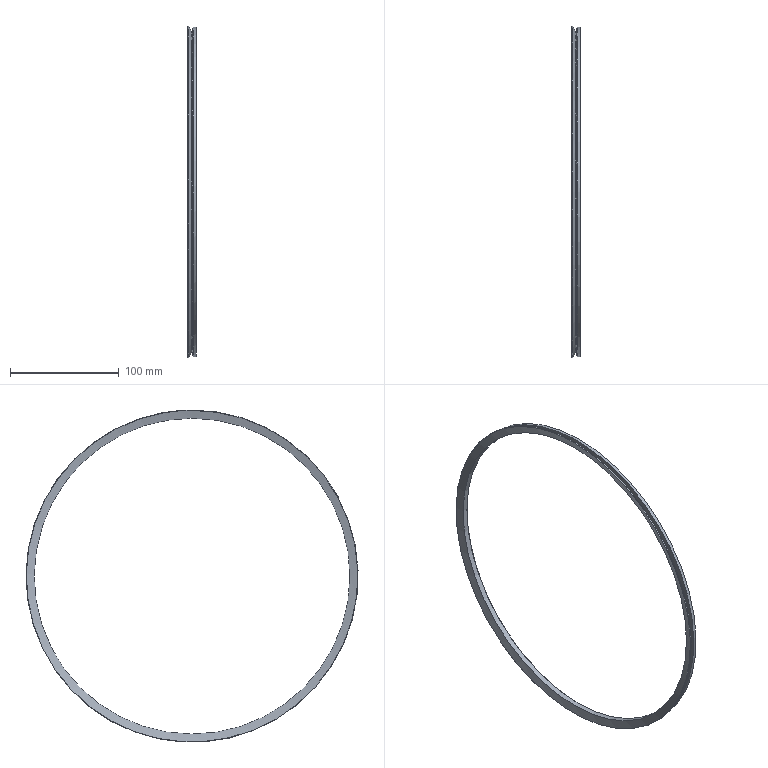Part | STEP file | Part [25] | 1 solid | 9 faces | box 8 x 304.945 x 304.945 mm | volume 31163 mm3 | cone 5 | cylinder 2 | torus 1 | plane 1 | commonest cylinder face diameters 290 x1 303 x1
STEP:
#1=CARTESIAN_POINT('',(4.567,0.,146.546));
#2=VERTEX_POINT('',#1);
#3=CARTESIAN_POINT('',(4.567,146.546,0.));
#4=VERTEX_POINT('',#3);
#5=CARTESIAN_POINT('',(4.567,0.,146.546));
#6=CARTESIAN_POINT('',(4.567,-3.07,146.546));
#7=CARTESIAN_POINT('',(4.567,-9.209,146.353));
#8=CARTESIAN_POINT('',(4.567,-18.382,145.486));
#9=CARTESIAN_POINT('',(4.567,-27.482,144.044));
#10=CARTESIAN_POINT('',(4.567,-36.474,142.034));
#11=CARTESIAN_POINT('',(4.567,-45.322,139.463));
#12=CARTESIAN_POINT('',(4.567,-53.991,136.341));
#13=CARTESIAN_POINT('',(4.567,-62.447,132.682));
#14=CARTESIAN_POINT('',(4.567,-70.656,128.498));
#15=CARTESIAN_POINT('',(4.567,-78.586,123.807));
#16=CARTESIAN_POINT('',(4.567,-86.206,118.628));
#17=CARTESIAN_POINT('',(4.567,-93.486,112.98));
#18=CARTESIAN_POINT('',(4.567,-100.397,106.886));
#19=CARTESIAN_POINT('',(4.567,-106.911,100.37));
#20=CARTESIAN_POINT('',(4.567,-113.003,93.458));
#21=CARTESIAN_POINT('',(4.567,-118.649,86.176));
#22=CARTESIAN_POINT('',(4.567,-123.827,78.555));
#23=CARTESIAN_POINT('',(4.567,-128.516,70.624));
#24=CARTESIAN_POINT('',(4.567,-132.697,62.413));
#25=CARTESIAN_POINT('',(4.567,-136.355,53.957));
#26=CARTESIAN_POINT('',(4.567,-139.474,45.287));
#27=CARTESIAN_POINT('',(4.567,-142.043,36.439));
#28=CARTESIAN_POINT('',(4.567,-144.051,27.446));
#29=CARTESIAN_POINT('',(4.567,-145.49,18.346));
#30=CARTESIAN_POINT('',(4.567,-146.354,9.185));
#31=CARTESIAN_POINT('',(4.567,-146.546,3.058));
#32=CARTESIAN_POINT('',(4.567,-146.546,0.));
#33=CARTESIAN_POINT('',(4.567,-146.546,-3.07));
#34=CARTESIAN_POINT('',(4.567,-146.353,-9.209));
#35=CARTESIAN_POINT('',(4.567,-145.486,-18.382));
#36=CARTESIAN_POINT('',(4.567,-144.044,-27.482));
#37=CARTESIAN_POINT('',(4.567,-142.034,-36.474));
#38=CARTESIAN_POINT('',(4.567,-139.463,-45.322));
#39=CARTESIAN_POINT('',(4.567,-136.341,-53.991));
#40=CARTESIAN_POINT('',(4.567,-132.682,-62.447));
#41=CARTESIAN_POINT('',(4.567,-128.498,-70.656));
#42=CARTESIAN_POINT('',(4.567,-123.807,-78.586));
#43=CARTESIAN_POINT('',(4.567,-118.628,-86.206));
#44=CARTESIAN_POINT('',(4.567,-112.98,-93.486));
#45=CARTESIAN_POINT('',(4.567,-106.886,-100.397));
#46=CARTESIAN_POINT('',(4.567,-100.37,-106.911));
#47=CARTESIAN_POINT('',(4.567,-93.458,-113.003));
#48=CARTESIAN_POINT('',(4.567,-86.176,-118.649));
#49=CARTESIAN_POINT('',(4.567,-78.555,-123.827));
#50=CARTESIAN_POINT('',(4.567,-70.624,-128.516));
#51=CARTESIAN_POINT('',(4.567,-62.413,-132.697));
#52=CARTESIAN_POINT('',(4.567,-53.957,-136.355));
#53=CARTESIAN_POINT('',(4.567,-45.287,-139.474));
#54=CARTESIAN_POINT('',(4.567,-36.439,-142.043));
#55=CARTESIAN_POINT('',(4.567,-27.446,-144.051));
#56=CARTESIAN_POINT('',(4.567,-18.346,-145.49));
#57=CARTESIAN_POINT('',(4.567,-9.173,-146.355));
#58=CARTESIAN_POINT('',(4.567,0.03666,-146.642));
#59=CARTESIAN_POINT('',(4.567,9.246,-146.351));
#60=CARTESIAN_POINT('',(4.567,18.418,-145.481));
#61=CARTESIAN_POINT('',(4.567,27.518,-144.037));
#62=CARTESIAN_POINT('',(4.567,36.51,-142.025));
#63=CARTESIAN_POINT('',(4.567,45.357,-139.452));
#64=CARTESIAN_POINT('',(4.567,54.025,-136.328));
#65=CARTESIAN_POINT('',(4.567,62.48,-132.666));
#66=CARTESIAN_POINT('',(4.567,70.688,-128.48));
#67=CARTESIAN_POINT('',(4.567,78.617,-123.788));
#68=CARTESIAN_POINT('',(4.567,86.236,-118.606));
#69=CARTESIAN_POINT('',(4.567,93.514,-112.956));
#70=CARTESIAN_POINT('',(4.567,100.423,-106.861));
#71=CARTESIAN_POINT('',(4.567,106.936,-100.343));
#72=CARTESIAN_POINT('',(4.567,113.026,-93.429));
#73=CARTESIAN_POINT('',(4.567,118.671,-86.147));
#74=CARTESIAN_POINT('',(4.567,123.847,-78.524));
#75=CARTESIAN_POINT('',(4.567,128.533,-70.592));
#76=CARTESIAN_POINT('',(4.567,132.713,-62.38));
#77=CARTESIAN_POINT('',(4.567,136.368,-53.923));
#78=CARTESIAN_POINT('',(4.567,139.486,-45.252));
#79=CARTESIAN_POINT('',(4.567,142.052,-36.403));
#80=CARTESIAN_POINT('',(4.567,144.058,-27.41));
#81=CARTESIAN_POINT('',(4.567,145.495,-18.309));
#82=CARTESIAN_POINT('',(4.567,146.355,-9.16));
#83=CARTESIAN_POINT('',(4.567,146.546,-3.045));
#84=CARTESIAN_POINT('',(4.567,146.546,0.));
#85=B_SPLINE_CURVE_WITH_KNOTS('',3,(#5,#6,#7,#8,#9,#10,#11,#12,#13,#14,#15,#16,#17,#18,#19,#20,#21,#22,#23,#24,#25,#26,#27,#28,#29,#30,#31,#32,#33,#34,#35,#36,#37,#38,#39,#40,#41,#42,#43,#44,#45,#46,#47,#48,#49,#50,#51,#52,#53,#54,#55,#56,#57,#58,#59,#60,#61,#62,#63,#64,#65,#66,#67,#68,#69,#70,#71,#72,#73,#74,#75,#76,#77,#78,#79,#80,#81,#82,#83,#84),.UNSPECIFIED.,.F.,.F.,(4,1,1,1,1,1,1,1,1,1,1,1,1,1,1,1,1,1,1,1,1,1,1,1,1,3,1,1,1,1,1,1,1,1,1,1,1,1,1,1,1,1,1,1,1,1,1,1,1,1,1,1,1,1,1,1,1,1,1,1,1,1,1,1,1,1,1,1,1,1,1,1,1,1,1,4),(0.,0.01334,0.02667,0.04001,0.05334,0.06668,0.08001,0.09335,0.1067,0.12,0.1334,0.1467,0.16,0.1734,0.1867,0.2,0.2134,0.2267,0.24,0.2534,0.2667,0.28,0.2934,0.3067,0.3201,0.3333,0.3467,0.36,0.3733,0.3867,0.4,0.4133,0.4267,0.44,0.4534,0.4667,0.48,0.4934,0.5067,0.52,0.5334,0.5467,0.56,0.5734,0.5867,0.6,0.6134,0.6267,0.64,0.6534,0.6667,0.6801,0.6934,0.7067,0.7201,0.7334,0.7467,0.7601,0.7734,0.7867,0.8001,0.8134,0.8267,0.8401,0.8534,0.8668,0.8801,0.8934,0.9068,0.9201,0.9334,0.9468,0.9601,0.9734,0.9868,1.),.UNSPECIFIED.);
#86=EDGE_CURVE('',#2,#4,#85,.T.);
#87=ORIENTED_EDGE('',*,*,#86,.F.);
#88=CARTESIAN_POINT('',(4.567,0.,0.));
#89=DIRECTION('',(1.,0.,0.));
#90=DIRECTION('',(0.,1.,0.));
#91=AXIS2_PLACEMENT_3D('',#88,#89,#90);
#92=CIRCLE('',#91,146.546);
#93=EDGE_CURVE('',#4,#2,#92,.T.);
#94=ORIENTED_EDGE('',*,*,#93,.F.);
#95=EDGE_LOOP('',(#87,#94));
#96=FACE_BOUND('',#95,.T.);
#97=CARTESIAN_POINT('',(3.61,146.39,0.));
#98=VERTEX_POINT('',#97);
#99=CARTESIAN_POINT('',(3.61,0.,146.39));
#100=VERTEX_POINT('',#99);
#101=CARTESIAN_POINT('',(3.61,0.,0.));
#102=DIRECTION('',(1.,0.,0.));
#103=DIRECTION('',(0.,1.,0.));
#104=AXIS2_PLACEMENT_3D('',#101,#102,#103);
#105=CIRCLE('',#104,146.39);
#106=EDGE_CURVE('',#98,#100,#105,.T.);
#107=ORIENTED_EDGE('',*,*,#106,.T.);
#108=CARTESIAN_POINT('',(3.61,0.,146.39));
#109=CARTESIAN_POINT('',(3.61,-3.066,146.39));
#110=CARTESIAN_POINT('',(3.61,-9.199,146.197));
#111=CARTESIAN_POINT('',(3.61,-18.363,145.331));
#112=CARTESIAN_POINT('',(3.61,-27.453,143.891));
#113=CARTESIAN_POINT('',(3.61,-36.435,141.883));
#114=CARTESIAN_POINT('',(3.61,-45.274,139.315));
#115=CARTESIAN_POINT('',(3.61,-53.933,136.196));
#116=CARTESIAN_POINT('',(3.61,-62.38,132.541));
#117=CARTESIAN_POINT('',(3.61,-70.581,128.361));
#118=CARTESIAN_POINT('',(3.61,-78.503,123.676));
#119=CARTESIAN_POINT('',(3.61,-86.114,118.501));
#120=CARTESIAN_POINT('',(3.61,-93.386,112.859));
#121=CARTESIAN_POINT('',(3.61,-100.29,106.772));
#122=CARTESIAN_POINT('',(3.61,-106.797,100.263));
#123=CARTESIAN_POINT('',(3.61,-112.883,93.358));
#124=CARTESIAN_POINT('',(3.61,-118.523,86.085));
#125=CARTESIAN_POINT('',(3.61,-123.695,78.472));
#126=CARTESIAN_POINT('',(3.61,-128.379,70.549));
#127=CARTESIAN_POINT('',(3.61,-132.556,62.347));
#128=CARTESIAN_POINT('',(3.61,-136.21,53.899));
#129=CARTESIAN_POINT('',(3.61,-139.326,45.239));
#130=CARTESIAN_POINT('',(3.61,-141.892,36.4));
#131=CARTESIAN_POINT('',(3.61,-143.898,27.417));
#132=CARTESIAN_POINT('',(3.61,-145.336,18.326));
#133=CARTESIAN_POINT('',(3.61,-146.2,9.163));
#134=CARTESIAN_POINT('',(3.61,-146.486,-0.03662));
#135=CARTESIAN_POINT('',(3.61,-146.195,-9.236));
#136=CARTESIAN_POINT('',(3.61,-145.326,-18.399));
#137=CARTESIAN_POINT('',(3.61,-143.884,-27.489));
#138=CARTESIAN_POINT('',(3.61,-141.874,-36.471));
#139=CARTESIAN_POINT('',(3.61,-139.303,-45.309));
#140=CARTESIAN_POINT('',(3.61,-136.183,-53.967));
#141=CARTESIAN_POINT('',(3.61,-132.525,-62.413));
#142=CARTESIAN_POINT('',(3.61,-128.344,-70.613));
#143=CARTESIAN_POINT('',(3.61,-123.656,-78.533));
#144=CARTESIAN_POINT('',(3.61,-118.48,-86.144));
#145=CARTESIAN_POINT('',(3.61,-112.836,-93.415));
#146=CARTESIAN_POINT('',(3.61,-106.747,-100.316));
#147=CARTESIAN_POINT('',(3.61,-100.236,-106.822));
#148=CARTESIAN_POINT('',(3.61,-93.33,-112.906));
#149=CARTESIAN_POINT('',(3.61,-86.055,-118.544));
#150=CARTESIAN_POINT('',(3.61,-78.441,-123.715));
#151=CARTESIAN_POINT('',(3.61,-70.516,-128.397));
#152=CARTESIAN_POINT('',(3.61,-62.314,-132.572));
#153=CARTESIAN_POINT('',(3.61,-53.865,-136.223));
#154=CARTESIAN_POINT('',(3.61,-45.204,-139.337));
#155=CARTESIAN_POINT('',(3.61,-36.364,-141.901));
#156=CARTESIAN_POINT('',(3.61,-27.381,-143.905));
#157=CARTESIAN_POINT('',(3.61,-18.29,-145.34));
#158=CARTESIAN_POINT('',(3.61,-9.151,-146.2));
#159=CARTESIAN_POINT('',(3.61,-3.042,-146.39));
#160=CARTESIAN_POINT('',(3.61,0.,-146.39));
#161=CARTESIAN_POINT('',(3.61,3.066,-146.39));
#162=CARTESIAN_POINT('',(3.61,9.199,-146.197));
#163=CARTESIAN_POINT('',(3.61,18.363,-145.331));
#164=CARTESIAN_POINT('',(3.61,27.453,-143.891));
#165=CARTESIAN_POINT('',(3.61,36.435,-141.883));
#166=CARTESIAN_POINT('',(3.61,45.274,-139.315));
#167=CARTESIAN_POINT('',(3.61,53.933,-136.196));
#168=CARTESIAN_POINT('',(3.61,62.38,-132.541));
#169=CARTESIAN_POINT('',(3.61,70.581,-128.361));
#170=CARTESIAN_POINT('',(3.61,78.503,-123.676));
#171=CARTESIAN_POINT('',(3.61,86.114,-118.501));
#172=CARTESIAN_POINT('',(3.61,93.386,-112.859));
#173=CARTESIAN_POINT('',(3.61,100.29,-106.772));
#174=CARTESIAN_POINT('',(3.61,106.797,-100.263));
#175=CARTESIAN_POINT('',(3.61,112.883,-93.358));
#176=CARTESIAN_POINT('',(3.61,118.523,-86.085));
#177=CARTESIAN_POINT('',(3.61,123.695,-78.472));
#178=CARTESIAN_POINT('',(3.61,128.379,-70.549));
#179=CARTESIAN_POINT('',(3.61,132.556,-62.347));
#180=CARTESIAN_POINT('',(3.61,136.21,-53.899));
#181=CARTESIAN_POINT('',(3.61,139.326,-45.239));
#182=CARTESIAN_POINT('',(3.61,141.892,-36.4));
#183=CARTESIAN_POINT('',(3.61,143.898,-27.417));
#184=CARTESIAN_POINT('',(3.61,145.336,-18.326));
#185=CARTESIAN_POINT('',(3.61,146.198,-9.175));
#186=CARTESIAN_POINT('',(3.61,146.39,-3.054));
#187=CARTESIAN_POINT('',(3.61,146.39,0.));
#188=B_SPLINE_CURVE_WITH_KNOTS('',3,(#108,#109,#110,#111,#112,#113,#114,#115,#116,#117,#118,#119,#120,#121,#122,#123,#124,#125,#126,#127,#128,#129,#130,#131,#132,#133,#134,#135,#136,#137,#138,#139,#140,#141,#142,#143,#144,#145,#146,#147,#148,#149,#150,#151,#152,#153,#154,#155,#156,#157,#158,#159,#160,#161,#162,#163,#164,#165,#166,#167,#168,#169,#170,#171,#172,#173,#174,#175,#176,#177,#178,#179,#180,#181,#182,#183,#184,#185,#186,#187),.UNSPECIFIED.,.F.,.F.,(4,1,1,1,1,1,1,1,1,1,1,1,1,1,1,1,1,1,1,1,1,1,1,1,1,1,1,1,1,1,1,1,1,1,1,1,1,1,1,1,1,1,1,1,1,1,1,1,1,1,3,1,1,1,1,1,1,1,1,1,1,1,1,1,1,1,1,1,1,1,1,1,1,1,1,4),(0.,0.01334,0.02667,0.04001,0.05334,0.06668,0.08001,0.09335,0.1067,0.12,0.1334,0.1467,0.16,0.1734,0.1867,0.2,0.2134,0.2267,0.24,0.2534,0.2667,0.28,0.2934,0.3067,0.3201,0.3334,0.3467,0.3601,0.3734,0.3867,0.4001,0.4134,0.4267,0.4401,0.4534,0.4667,0.4801,0.4934,0.5067,0.5201,0.5334,0.5468,0.5601,0.5734,0.5868,0.6001,0.6134,0.6268,0.6401,0.6534,0.6667,0.68,0.6933,0.7067,0.72,0.7333,0.7467,0.76,0.7734,0.7867,0.8,0.8134,0.8267,0.84,0.8534,0.8667,0.88,0.8934,0.9067,0.92,0.9334,0.9467,0.96,0.9734,0.9867,1.),.UNSPECIFIED.);
#189=EDGE_CURVE('',#100,#98,#188,.T.);
#190=ORIENTED_EDGE('',*,*,#189,.T.);
#191=EDGE_LOOP('',(#107,#190));
#192=FACE_BOUND('',#191,.T.);
#193=CARTESIAN_POINT('',(4.069,0.,0.));
#194=DIRECTION('',(1.,0.,0.));
#195=DIRECTION('',(0.,1.,0.));
#196=AXIS2_PLACEMENT_3D('',#193,#194,#195);
#197=TOROIDAL_SURFACE('',#196,146.59,0.5);
#198=ADVANCED_FACE('',(#96,#192),#197,.F.);
#199=CARTESIAN_POINT('',(8.,0.,146.));
#200=VERTEX_POINT('',#199);
#201=CARTESIAN_POINT('',(8.,0.,0.));
#202=DIRECTION('',(1.,0.,0.));
#203=DIRECTION('',(0.,0.,-1.));
#204=AXIS2_PLACEMENT_3D('',#201,#202,#203);
#205=CIRCLE('',#204,146.);
#206=EDGE_CURVE('',#200,#200,#205,.T.);
#207=ORIENTED_EDGE('',*,*,#206,.T.);
#208=EDGE_LOOP('',(#207));
#209=FACE_OUTER_BOUND('',#208,.T.);
#210=CARTESIAN_POINT('',(7.,0.,145.));
#211=VERTEX_POINT('',#210);
#212=CARTESIAN_POINT('',(7.,0.,145.));
#213=CARTESIAN_POINT('',(7.,-3.037,145.));
#214=CARTESIAN_POINT('',(7.,-9.112,144.809));
#215=CARTESIAN_POINT('',(7.,-18.188,143.951));
#216=CARTESIAN_POINT('',(7.,-27.192,142.525));
#217=CARTESIAN_POINT('',(7.,-36.089,140.536));
#218=CARTESIAN_POINT('',(7.,-44.844,137.992));
#219=CARTESIAN_POINT('',(7.,-53.421,134.903));
#220=CARTESIAN_POINT('',(7.,-61.788,131.282));
#221=CARTESIAN_POINT('',(7.,-69.91,127.143));
#222=CARTESIAN_POINT('',(7.,-77.757,122.501));
#223=CARTESIAN_POINT('',(7.,-85.297,117.376));
#224=CARTESIAN_POINT('',(7.,-92.5,111.788));
#225=CARTESIAN_POINT('',(7.,-99.337,105.758));
#226=CARTESIAN_POINT('',(7.,-105.783,99.311));
#227=CARTESIAN_POINT('',(7.,-111.811,92.472));
#228=CARTESIAN_POINT('',(7.,-117.397,85.267));
#229=CARTESIAN_POINT('',(7.,-122.521,77.726));
#230=CARTESIAN_POINT('',(7.,-127.16,69.879));
#231=CARTESIAN_POINT('',(7.,-131.297,61.755));
#232=CARTESIAN_POINT('',(7.,-134.917,53.388));
#233=CARTESIAN_POINT('',(7.,-138.003,44.809));
#234=CARTESIAN_POINT('',(7.,-140.545,36.054));
#235=CARTESIAN_POINT('',(7.,-142.531,27.157));
#236=CARTESIAN_POINT('',(7.,-143.956,18.152));
#237=CARTESIAN_POINT('',(7.,-144.811,9.076));
#238=CARTESIAN_POINT('',(7.,-145.095,-0.03627));
#239=CARTESIAN_POINT('',(7.,-144.807,-9.148));
#240=CARTESIAN_POINT('',(7.,-143.946,-18.224));
#241=CARTESIAN_POINT('',(7.,-142.518,-27.228));
#242=CARTESIAN_POINT('',(7.,-140.527,-36.125));
#243=CARTESIAN_POINT('',(7.,-137.981,-44.878));
#244=CARTESIAN_POINT('',(7.,-134.89,-53.455));
#245=CARTESIAN_POINT('',(7.,-131.267,-61.821));
#246=CARTESIAN_POINT('',(7.,-127.125,-69.942));
#247=CARTESIAN_POINT('',(7.,-122.482,-77.788));
#248=CARTESIAN_POINT('',(7.,-117.355,-85.326));
#249=CARTESIAN_POINT('',(7.,-111.765,-92.528));
#250=CARTESIAN_POINT('',(7.,-105.733,-99.364));
#251=CARTESIAN_POINT('',(7.,-99.284,-105.808));
#252=CARTESIAN_POINT('',(7.,-92.444,-111.834));
#253=CARTESIAN_POINT('',(7.,-85.238,-117.419));
#254=CARTESIAN_POINT('',(7.,-77.696,-122.54));
#255=CARTESIAN_POINT('',(7.,-69.847,-127.177));
#256=CARTESIAN_POINT('',(7.,-61.722,-131.313));
#257=CARTESIAN_POINT('',(7.,-53.354,-134.93));
#258=CARTESIAN_POINT('',(7.,-44.775,-138.014));
#259=CARTESIAN_POINT('',(7.,-36.019,-140.554));
#260=CARTESIAN_POINT('',(7.,-27.121,-142.538));
#261=CARTESIAN_POINT('',(7.,-18.116,-143.96));
#262=CARTESIAN_POINT('',(7.,-9.064,-144.811));
#263=CARTESIAN_POINT('',(7.,-3.013,-145.));
#264=CARTESIAN_POINT('',(7.,0.,-145.));
#265=CARTESIAN_POINT('',(7.,3.037,-145.));
#266=CARTESIAN_POINT('',(7.,9.112,-144.809));
#267=CARTESIAN_POINT('',(7.,18.188,-143.951));
#268=CARTESIAN_POINT('',(7.,27.192,-142.525));
#269=CARTESIAN_POINT('',(7.,36.089,-140.536));
#270=CARTESIAN_POINT('',(7.,44.844,-137.992));
#271=CARTESIAN_POINT('',(7.,53.421,-134.903));
#272=CARTESIAN_POINT('',(7.,61.788,-131.282));
#273=CARTESIAN_POINT('',(7.,69.91,-127.143));
#274=CARTESIAN_POINT('',(7.,77.757,-122.501));
#275=CARTESIAN_POINT('',(7.,85.297,-117.376));
#276=CARTESIAN_POINT('',(7.,92.5,-111.788));
#277=CARTESIAN_POINT('',(7.,99.337,-105.758));
#278=CARTESIAN_POINT('',(7.,105.783,-99.311));
#279=CARTESIAN_POINT('',(7.,111.811,-92.472));
#280=CARTESIAN_POINT('',(7.,117.397,-85.267));
#281=CARTESIAN_POINT('',(7.,122.521,-77.726));
#282=CARTESIAN_POINT('',(7.,127.16,-69.879));
#283=CARTESIAN_POINT('',(7.,131.297,-61.755));
#284=CARTESIAN_POINT('',(7.,134.917,-53.388));
#285=CARTESIAN_POINT('',(7.,138.003,-44.809));
#286=CARTESIAN_POINT('',(7.,140.545,-36.054));
#287=CARTESIAN_POINT('',(7.,142.531,-27.157));
#288=CARTESIAN_POINT('',(7.,143.956,-18.152));
#289=CARTESIAN_POINT('',(7.,144.811,-9.076));
#290=CARTESIAN_POINT('',(7.,145.095,0.03627));
#291=CARTESIAN_POINT('',(7.,144.807,9.148));
#292=CARTESIAN_POINT('',(7.,143.946,18.224));
#293=CARTESIAN_POINT('',(7.,142.518,27.228));
#294=CARTESIAN_POINT('',(7.,140.527,36.125));
#295=CARTESIAN_POINT('',(7.,137.981,44.878));
#296=CARTESIAN_POINT('',(7.,134.89,53.455));
#297=CARTESIAN_POINT('',(7.,131.267,61.821));
#298=CARTESIAN_POINT('',(7.,127.125,69.942));
#299=CARTESIAN_POINT('',(7.,122.482,77.788));
#300=CARTESIAN_POINT('',(7.,117.355,85.326));
#301=CARTESIAN_POINT('',(7.,111.765,92.528));
#302=CARTESIAN_POINT('',(7.,105.733,99.364));
#303=CARTESIAN_POINT('',(7.,99.284,105.808));
#304=CARTESIAN_POINT('',(7.,92.444,111.834));
#305=CARTESIAN_POINT('',(7.,85.238,117.419));
#306=CARTESIAN_POINT('',(7.,77.696,122.54));
#307=CARTESIAN_POINT('',(7.,69.847,127.177));
#308=CARTESIAN_POINT('',(7.,61.722,131.313));
#309=CARTESIAN_POINT('',(7.,53.354,134.93));
#310=CARTESIAN_POINT('',(7.,44.775,138.014));
#311=CARTESIAN_POINT('',(7.,36.019,140.554));
#312=CARTESIAN_POINT('',(7.,27.121,142.538));
#313=CARTESIAN_POINT('',(7.,18.116,143.96));
#314=CARTESIAN_POINT('',(7.,9.064,144.811));
#315=CARTESIAN_POINT('',(7.,3.013,145.));
#316=CARTESIAN_POINT('',(7.,0.,145.));
#317=B_SPLINE_CURVE_WITH_KNOTS('',3,(#212,#213,#214,#215,#216,#217,#218,#219,#220,#221,#222,#223,#224,#225,#226,#227,#228,#229,#230,#231,#232,#233,#234,#235,#236,#237,#238,#239,#240,#241,#242,#243,#244,#245,#246,#247,#248,#249,#250,#251,#252,#253,#254,#255,#256,#257,#258,#259,#260,#261,#262,#263,#264,#265,#266,#267,#268,#269,#270,#271,#272,#273,#274,#275,#276,#277,#278,#279,#280,#281,#282,#283,#284,#285,#286,#287,#288,#289,#290,#291,#292,#293,#294,#295,#296,#297,#298,#299,#300,#301,#302,#303,#304,#305,#306,#307,#308,#309,#310,#311,#312,#313,#314,#315,#316),.UNSPECIFIED.,.T.,.F.,(4,1,1,1,1,1,1,1,1,1,1,1,1,1,1,1,1,1,1,1,1,1,1,1,1,1,1,1,1,1,1,1,1,1,1,1,1,1,1,1,1,1,1,1,1,1,1,1,1,1,3,1,1,1,1,1,1,1,1,1,1,1,1,1,1,1,1,1,1,1,1,1,1,1,1,1,1,1,1,1,1,1,1,1,1,1,1,1,1,1,1,1,1,1,1,1,1,1,1,1,4),(0.,0.01,0.02,0.03,0.04001,0.05001,0.06001,0.07001,0.08001,0.09001,0.1,0.11,0.12,0.13,0.14,0.15,0.16,0.17,0.18,0.19,0.2,0.21,0.22,0.23,0.24,0.25,0.26,0.27,0.28,0.29,0.3,0.31,0.3201,0.3301,0.3401,0.3501,0.3601,0.3701,0.3801,0.3901,0.4001,0.4101,0.4201,0.4301,0.4401,0.4501,0.4601,0.4701,0.4801,0.4901,0.5,0.51,0.52,0.53,0.54,0.55,0.56,0.57,0.58,0.59,0.6,0.61,0.62,0.63,0.64,0.65,0.66,0.67,0.68,0.69,0.7,0.71,0.72,0.73,0.74,0.75,0.76,0.77,0.78,0.79,0.8,0.81,0.8201,0.8301,0.8401,0.8501,0.8601,0.8701,0.8801,0.8901,0.9001,0.9101,0.9201,0.9301,0.9401,0.9501,0.9601,0.9701,0.9801,0.9901,1.),.UNSPECIFIED.);
#318=EDGE_CURVE('',#211,#211,#317,.T.);
#319=ORIENTED_EDGE('',*,*,#318,.F.);
#320=EDGE_LOOP('',(#319));
#321=FACE_OUTER_BOUND('',#320,.T.);
#322=CARTESIAN_POINT('',(7.5,0.,0.));
#323=DIRECTION('',(1.,0.,0.));
#324=DIRECTION('',(0.,0.,1.));
#325=AXIS2_PLACEMENT_3D('',#322,#323,#324);
#326=CONICAL_SURFACE('',#325,145.5,0.7854);
#327=ADVANCED_FACE('',(#209,#321),#326,.F.);
#328=CARTESIAN_POINT('',(8.,0.,151.5));
#329=VERTEX_POINT('',#328);
#330=CARTESIAN_POINT('',(8.,0.,0.));
#331=DIRECTION('',(1.,0.,0.));
#332=DIRECTION('',(0.,0.,1.));
#333=AXIS2_PLACEMENT_3D('',#330,#331,#332);
#334=CIRCLE('',#333,151.5);
#335=EDGE_CURVE('',#329,#329,#334,.T.);
#336=ORIENTED_EDGE('',*,*,#335,.F.);
#337=EDGE_LOOP('',(#336));
#338=FACE_OUTER_BOUND('',#337,.T.);
#339=CARTESIAN_POINT('',(5.,0.,151.5));
#340=VERTEX_POINT('',#339);
#341=CARTESIAN_POINT('',(5.,0.,151.5));
#342=CARTESIAN_POINT('',(5.,-3.174,151.5));
#343=CARTESIAN_POINT('',(5.,-9.521,151.3));
#344=CARTESIAN_POINT('',(5.,-19.003,150.404));
#345=CARTESIAN_POINT('',(5.,-28.411,148.914));
#346=CARTESIAN_POINT('',(5.,-37.707,146.835));
#347=CARTESIAN_POINT('',(5.,-46.854,144.178));
#348=CARTESIAN_POINT('',(5.,-55.816,140.951));
#349=CARTESIAN_POINT('',(5.,-64.558,137.167));
#350=CARTESIAN_POINT('',(5.,-73.044,132.842));
#351=CARTESIAN_POINT('',(5.,-81.243,127.993));
#352=CARTESIAN_POINT('',(5.,-89.12,122.638));
#353=CARTESIAN_POINT('',(5.,-96.646,116.799));
#354=CARTESIAN_POINT('',(5.,-103.79,110.499));
#355=CARTESIAN_POINT('',(5.,-110.525,103.763));
#356=CARTESIAN_POINT('',(5.,-116.823,96.617));
#357=CARTESIAN_POINT('',(5.,-122.66,89.09));
#358=CARTESIAN_POINT('',(5.,-128.013,81.211));
#359=CARTESIAN_POINT('',(5.,-132.86,73.011));
#360=CARTESIAN_POINT('',(5.,-137.183,64.523));
#361=CARTESIAN_POINT('',(5.,-140.964,55.781));
#362=CARTESIAN_POINT('',(5.,-144.189,46.818));
#363=CARTESIAN_POINT('',(5.,-146.845,37.67));
#364=CARTESIAN_POINT('',(5.,-148.921,28.374));
#365=CARTESIAN_POINT('',(5.,-150.409,18.966));
#366=CARTESIAN_POINT('',(5.,-151.303,9.483));
#367=CARTESIAN_POINT('',(5.,-151.6,-0.0379));
#368=CARTESIAN_POINT('',(5.,-151.298,-9.558));
#369=CARTESIAN_POINT('',(5.,-150.399,-19.041));
#370=CARTESIAN_POINT('',(5.,-148.907,-28.449));
#371=CARTESIAN_POINT('',(5.,-146.826,-37.744));
#372=CARTESIAN_POINT('',(5.,-144.166,-46.89));
#373=CARTESIAN_POINT('',(5.,-140.937,-55.851));
#374=CARTESIAN_POINT('',(5.,-137.151,-64.592));
#375=CARTESIAN_POINT('',(5.,-132.824,-73.078));
#376=CARTESIAN_POINT('',(5.,-127.972,-81.275));
#377=CARTESIAN_POINT('',(5.,-122.616,-89.151));
#378=CARTESIAN_POINT('',(5.,-116.775,-96.675));
#379=CARTESIAN_POINT('',(5.,-110.473,-103.818));
#380=CARTESIAN_POINT('',(5.,-103.735,-110.551));
#381=CARTESIAN_POINT('',(5.,-96.588,-116.847));
#382=CARTESIAN_POINT('',(5.,-89.059,-122.682));
#383=CARTESIAN_POINT('',(5.,-81.179,-128.033));
#384=CARTESIAN_POINT('',(5.,-72.978,-132.879));
#385=CARTESIAN_POINT('',(5.,-64.489,-137.199));
#386=CARTESIAN_POINT('',(5.,-55.746,-140.978));
#387=CARTESIAN_POINT('',(5.,-46.782,-144.201));
#388=CARTESIAN_POINT('',(5.,-37.634,-146.854));
#389=CARTESIAN_POINT('',(5.,-28.337,-148.928));
#390=CARTESIAN_POINT('',(5.,-18.928,-150.413));
#391=CARTESIAN_POINT('',(5.,-9.47,-151.303));
#392=CARTESIAN_POINT('',(5.,-3.148,-151.5));
#393=CARTESIAN_POINT('',(5.,0.,-151.5));
#394=CARTESIAN_POINT('',(5.,3.174,-151.5));
#395=CARTESIAN_POINT('',(5.,9.521,-151.3));
#396=CARTESIAN_POINT('',(5.,19.003,-150.404));
#397=CARTESIAN_POINT('',(5.,28.411,-148.914));
#398=CARTESIAN_POINT('',(5.,37.707,-146.835));
#399=CARTESIAN_POINT('',(5.,46.854,-144.178));
#400=CARTESIAN_POINT('',(5.,55.816,-140.951));
#401=CARTESIAN_POINT('',(5.,64.558,-137.167));
#402=CARTESIAN_POINT('',(5.,73.044,-132.842));
#403=CARTESIAN_POINT('',(5.,81.243,-127.993));
#404=CARTESIAN_POINT('',(5.,89.12,-122.638));
#405=CARTESIAN_POINT('',(5.,96.646,-116.799));
#406=CARTESIAN_POINT('',(5.,103.79,-110.499));
#407=CARTESIAN_POINT('',(5.,110.525,-103.763));
#408=CARTESIAN_POINT('',(5.,116.823,-96.617));
#409=CARTESIAN_POINT('',(5.,122.66,-89.09));
#410=CARTESIAN_POINT('',(5.,128.013,-81.211));
#411=CARTESIAN_POINT('',(5.,132.86,-73.011));
#412=CARTESIAN_POINT('',(5.,137.183,-64.523));
#413=CARTESIAN_POINT('',(5.,140.964,-55.781));
#414=CARTESIAN_POINT('',(5.,144.189,-46.818));
#415=CARTESIAN_POINT('',(5.,146.845,-37.67));
#416=CARTESIAN_POINT('',(5.,148.921,-28.374));
#417=CARTESIAN_POINT('',(5.,150.409,-18.966));
#418=CARTESIAN_POINT('',(5.,151.303,-9.483));
#419=CARTESIAN_POINT('',(5.,151.6,0.0379));
#420=CARTESIAN_POINT('',(5.,151.298,9.558));
#421=CARTESIAN_POINT('',(5.,150.399,19.041));
#422=CARTESIAN_POINT('',(5.,148.907,28.449));
#423=CARTESIAN_POINT('',(5.,146.826,37.744));
#424=CARTESIAN_POINT('',(5.,144.166,46.89));
#425=CARTESIAN_POINT('',(5.,140.937,55.851));
#426=CARTESIAN_POINT('',(5.,137.151,64.592));
#427=CARTESIAN_POINT('',(5.,132.824,73.078));
#428=CARTESIAN_POINT('',(5.,127.972,81.275));
#429=CARTESIAN_POINT('',(5.,122.616,89.151));
#430=CARTESIAN_POINT('',(5.,116.775,96.675));
#431=CARTESIAN_POINT('',(5.,110.473,103.818));
#432=CARTESIAN_POINT('',(5.,103.735,110.551));
#433=CARTESIAN_POINT('',(5.,96.588,116.847));
#434=CARTESIAN_POINT('',(5.,89.059,122.682));
#435=CARTESIAN_POINT('',(5.,81.179,128.033));
#436=CARTESIAN_POINT('',(5.,72.978,132.879));
#437=CARTESIAN_POINT('',(5.,64.489,137.199));
#438=CARTESIAN_POINT('',(5.,55.746,140.978));
#439=CARTESIAN_POINT('',(5.,46.782,144.201));
#440=CARTESIAN_POINT('',(5.,37.634,146.854));
#441=CARTESIAN_POINT('',(5.,28.337,148.928));
#442=CARTESIAN_POINT('',(5.,18.928,150.413));
#443=CARTESIAN_POINT('',(5.,9.47,151.303));
#444=CARTESIAN_POINT('',(5.,3.148,151.5));
#445=CARTESIAN_POINT('',(5.,0.,151.5));
#446=B_SPLINE_CURVE_WITH_KNOTS('',3,(#341,#342,#343,#344,#345,#346,#347,#348,#349,#350,#351,#352,#353,#354,#355,#356,#357,#358,#359,#360,#361,#362,#363,#364,#365,#366,#367,#368,#369,#370,#371,#372,#373,#374,#375,#376,#377,#378,#379,#380,#381,#382,#383,#384,#385,#386,#387,#388,#389,#390,#391,#392,#393,#394,#395,#396,#397,#398,#399,#400,#401,#402,#403,#404,#405,#406,#407,#408,#409,#410,#411,#412,#413,#414,#415,#416,#417,#418,#419,#420,#421,#422,#423,#424,#425,#426,#427,#428,#429,#430,#431,#432,#433,#434,#435,#436,#437,#438,#439,#440,#441,#442,#443,#444,#445),.UNSPECIFIED.,.T.,.F.,(4,1,1,1,1,1,1,1,1,1,1,1,1,1,1,1,1,1,1,1,1,1,1,1,1,1,1,1,1,1,1,1,1,1,1,1,1,1,1,1,1,1,1,1,1,1,1,1,1,1,3,1,1,1,1,1,1,1,1,1,1,1,1,1,1,1,1,1,1,1,1,1,1,1,1,1,1,1,1,1,1,1,1,1,1,1,1,1,1,1,1,1,1,1,1,1,1,1,1,1,4),(0.,0.01,0.02,0.03,0.04001,0.05001,0.06001,0.07001,0.08001,0.09001,0.1,0.11,0.12,0.13,0.14,0.15,0.16,0.17,0.18,0.19,0.2,0.21,0.22,0.23,0.24,0.25,0.26,0.27,0.28,0.29,0.3,0.31,0.3201,0.3301,0.3401,0.3501,0.3601,0.3701,0.3801,0.3901,0.4001,0.4101,0.4201,0.4301,0.4401,0.4501,0.4601,0.4701,0.4801,0.4901,0.5,0.51,0.52,0.53,0.54,0.55,0.56,0.57,0.58,0.59,0.6,0.61,0.62,0.63,0.64,0.65,0.66,0.67,0.68,0.69,0.7,0.71,0.72,0.73,0.74,0.75,0.76,0.77,0.78,0.79,0.8,0.81,0.8201,0.8301,0.8401,0.8501,0.8601,0.8701,0.8801,0.8901,0.9001,0.9101,0.9201,0.9301,0.9401,0.9501,0.9601,0.9701,0.9801,0.9901,1.),.UNSPECIFIED.);
#447=EDGE_CURVE('',#340,#340,#446,.T.);
#448=ORIENTED_EDGE('',*,*,#447,.T.);
#449=EDGE_LOOP('',(#448));
#450=FACE_OUTER_BOUND('',#449,.T.);
#451=CARTESIAN_POINT('',(6.5,0.,0.));
#452=DIRECTION('',(1.,0.,0.));
#453=DIRECTION('',(0.,0.,1.));
#454=AXIS2_PLACEMENT_3D('',#451,#452,#453);
#455=CYLINDRICAL_SURFACE('',#454,151.5);
#456=ADVANCED_FACE('',(#338,#450),#455,.T.);
#457=ORIENTED_EDGE('',*,*,#447,.F.);
#458=EDGE_LOOP('',(#457));
#459=FACE_OUTER_BOUND('',#458,.T.);
#460=ORIENTED_EDGE('',*,*,#93,.T.);
#461=ORIENTED_EDGE('',*,*,#86,.T.);
#462=EDGE_LOOP('',(#460,#461));
#463=FACE_BOUND('',#462,.T.);
#464=CARTESIAN_POINT('',(4.783,0.,0.));
#465=DIRECTION('',(1.,0.,0.));
#466=DIRECTION('',(0.,0.,1.));
#467=AXIS2_PLACEMENT_3D('',#464,#465,#466);
#468=CONICAL_SURFACE('',#467,149.023,1.484);
#469=ADVANCED_FACE('',(#459,#463),#468,.T.);
#470=ORIENTED_EDGE('',*,*,#189,.F.);
#471=ORIENTED_EDGE('',*,*,#106,.F.);
#472=EDGE_LOOP('',(#470,#471));
#473=FACE_BOUND('',#472,.T.);
#474=CARTESIAN_POINT('',(0.9636,0.,152.472));
#475=VERTEX_POINT('',#474);
#476=CARTESIAN_POINT('',(0.9636,0.,152.472));
#477=CARTESIAN_POINT('',(0.9636,-3.194,152.473));
#478=CARTESIAN_POINT('',(0.9636,-9.582,152.272));
#479=CARTESIAN_POINT('',(0.9636,-19.125,151.369));
#480=CARTESIAN_POINT('',(0.9636,-28.594,149.869));
#481=CARTESIAN_POINT('',(0.9636,-37.949,147.778));
#482=CARTESIAN_POINT('',(0.9636,-47.155,145.103));
#483=CARTESIAN_POINT('',(0.9636,-56.174,141.855));
#484=CARTESIAN_POINT('',(0.9636,-64.972,138.047));
#485=CARTESIAN_POINT('',(0.9636,-73.513,133.695));
#486=CARTESIAN_POINT('',(0.9636,-81.764,128.814));
#487=CARTESIAN_POINT('',(0.9636,-89.692,123.425));
#488=CARTESIAN_POINT('',(0.9636,-97.266,117.549));
#489=CARTESIAN_POINT('',(0.9636,-104.457,111.208));
#490=CARTESIAN_POINT('',(0.9636,-111.234,104.429));
#491=CARTESIAN_POINT('',(0.9636,-117.573,97.237));
#492=CARTESIAN_POINT('',(0.9636,-123.447,89.662));
#493=CARTESIAN_POINT('',(0.9636,-128.835,81.732));
#494=CARTESIAN_POINT('',(0.9636,-133.713,73.48));
#495=CARTESIAN_POINT('',(0.9636,-138.064,64.937));
#496=CARTESIAN_POINT('',(0.9636,-141.869,56.139));
#497=CARTESIAN_POINT('',(0.9636,-145.115,47.119));
#498=CARTESIAN_POINT('',(0.9636,-147.787,37.912));
#499=CARTESIAN_POINT('',(0.9636,-149.877,28.556));
#500=CARTESIAN_POINT('',(0.9636,-151.374,19.088));
#501=CARTESIAN_POINT('',(0.9636,-152.274,9.544));
#502=CARTESIAN_POINT('',(0.9636,-152.573,-0.03814));
#503=CARTESIAN_POINT('',(0.9636,-152.269,-9.62));
#504=CARTESIAN_POINT('',(0.9636,-151.365,-19.163));
#505=CARTESIAN_POINT('',(0.9636,-149.862,-28.631));
#506=CARTESIAN_POINT('',(0.9636,-147.768,-37.986));
#507=CARTESIAN_POINT('',(0.9636,-145.091,-47.191));
#508=CARTESIAN_POINT('',(0.9636,-141.841,-56.21));
#509=CARTESIAN_POINT('',(0.9636,-138.031,-65.007));
#510=CARTESIAN_POINT('',(0.9636,-133.676,-73.547));
#511=CARTESIAN_POINT('',(0.9636,-128.794,-81.796));
#512=CARTESIAN_POINT('',(0.9636,-123.403,-89.723));
#513=CARTESIAN_POINT('',(0.9636,-117.524,-97.296));
#514=CARTESIAN_POINT('',(0.9636,-111.182,-104.484));
#515=CARTESIAN_POINT('',(0.9636,-104.401,-111.26));
#516=CARTESIAN_POINT('',(0.9636,-97.208,-117.597));
#517=CARTESIAN_POINT('',(0.9636,-89.631,-123.47));
#518=CARTESIAN_POINT('',(0.9636,-81.7,-128.855));
#519=CARTESIAN_POINT('',(0.9636,-73.446,-133.731));
#520=CARTESIAN_POINT('',(0.9636,-64.903,-138.08));
#521=CARTESIAN_POINT('',(0.9636,-56.103,-141.883));
#522=CARTESIAN_POINT('',(0.9636,-47.082,-145.127));
#523=CARTESIAN_POINT('',(0.9636,-37.875,-147.797));
#524=CARTESIAN_POINT('',(0.9636,-28.519,-149.884));
#525=CARTESIAN_POINT('',(0.9636,-19.05,-151.379));
#526=CARTESIAN_POINT('',(0.9636,-9.531,-152.274));
#527=CARTESIAN_POINT('',(0.9636,-3.168,-152.473));
#528=CARTESIAN_POINT('',(0.9636,0.,-152.472));
#529=CARTESIAN_POINT('',(0.9636,3.194,-152.473));
#530=CARTESIAN_POINT('',(0.9636,9.582,-152.272));
#531=CARTESIAN_POINT('',(0.9636,19.125,-151.369));
#532=CARTESIAN_POINT('',(0.9636,28.594,-149.869));
#533=CARTESIAN_POINT('',(0.9636,37.949,-147.778));
#534=CARTESIAN_POINT('',(0.9636,47.155,-145.103));
#535=CARTESIAN_POINT('',(0.9636,56.174,-141.855));
#536=CARTESIAN_POINT('',(0.9636,64.972,-138.047));
#537=CARTESIAN_POINT('',(0.9636,73.513,-133.695));
#538=CARTESIAN_POINT('',(0.9636,81.764,-128.814));
#539=CARTESIAN_POINT('',(0.9636,89.692,-123.425));
#540=CARTESIAN_POINT('',(0.9636,97.266,-117.549));
#541=CARTESIAN_POINT('',(0.9636,104.457,-111.208));
#542=CARTESIAN_POINT('',(0.9636,111.234,-104.429));
#543=CARTESIAN_POINT('',(0.9636,117.573,-97.237));
#544=CARTESIAN_POINT('',(0.9636,123.447,-89.662));
#545=CARTESIAN_POINT('',(0.9636,128.835,-81.732));
#546=CARTESIAN_POINT('',(0.9636,133.713,-73.48));
#547=CARTESIAN_POINT('',(0.9636,138.064,-64.937));
#548=CARTESIAN_POINT('',(0.9636,141.869,-56.139));
#549=CARTESIAN_POINT('',(0.9636,145.115,-47.119));
#550=CARTESIAN_POINT('',(0.9636,147.787,-37.912));
#551=CARTESIAN_POINT('',(0.9636,149.877,-28.556));
#552=CARTESIAN_POINT('',(0.9636,151.374,-19.088));
#553=CARTESIAN_POINT('',(0.9636,152.274,-9.544));
#554=CARTESIAN_POINT('',(0.9636,152.573,0.03814));
#555=CARTESIAN_POINT('',(0.9636,152.269,9.62));
#556=CARTESIAN_POINT('',(0.9636,151.365,19.163));
#557=CARTESIAN_POINT('',(0.9636,149.862,28.631));
#558=CARTESIAN_POINT('',(0.9636,147.768,37.986));
#559=CARTESIAN_POINT('',(0.9636,145.091,47.191));
#560=CARTESIAN_POINT('',(0.9636,141.841,56.21));
#561=CARTESIAN_POINT('',(0.9636,138.031,65.007));
#562=CARTESIAN_POINT('',(0.9636,133.676,73.547));
#563=CARTESIAN_POINT('',(0.9636,128.794,81.796));
#564=CARTESIAN_POINT('',(0.9636,123.403,89.723));
#565=CARTESIAN_POINT('',(0.9636,117.524,97.296));
#566=CARTESIAN_POINT('',(0.9636,111.182,104.484));
#567=CARTESIAN_POINT('',(0.9636,104.401,111.26));
#568=CARTESIAN_POINT('',(0.9636,97.208,117.597));
#569=CARTESIAN_POINT('',(0.9636,89.631,123.47));
#570=CARTESIAN_POINT('',(0.9636,81.7,128.855));
#571=CARTESIAN_POINT('',(0.9636,73.446,133.731));
#572=CARTESIAN_POINT('',(0.9636,64.903,138.08));
#573=CARTESIAN_POINT('',(0.9636,56.103,141.883));
#574=CARTESIAN_POINT('',(0.9636,47.082,145.127));
#575=CARTESIAN_POINT('',(0.9636,37.875,147.797));
#576=CARTESIAN_POINT('',(0.9636,28.519,149.884));
#577=CARTESIAN_POINT('',(0.9636,19.05,151.379));
#578=CARTESIAN_POINT('',(0.9636,9.531,152.274));
#579=CARTESIAN_POINT('',(0.9636,3.168,152.473));
#580=CARTESIAN_POINT('',(0.9636,0.,152.472));
#581=B_SPLINE_CURVE_WITH_KNOTS('',3,(#476,#477,#478,#479,#480,#481,#482,#483,#484,#485,#486,#487,#488,#489,#490,#491,#492,#493,#494,#495,#496,#497,#498,#499,#500,#501,#502,#503,#504,#505,#506,#507,#508,#509,#510,#511,#512,#513,#514,#515,#516,#517,#518,#519,#520,#521,#522,#523,#524,#525,#526,#527,#528,#529,#530,#531,#532,#533,#534,#535,#536,#537,#538,#539,#540,#541,#542,#543,#544,#545,#546,#547,#548,#549,#550,#551,#552,#553,#554,#555,#556,#557,#558,#559,#560,#561,#562,#563,#564,#565,#566,#567,#568,#569,#570,#571,#572,#573,#574,#575,#576,#577,#578,#579,#580),.UNSPECIFIED.,.T.,.F.,(4,1,1,1,1,1,1,1,1,1,1,1,1,1,1,1,1,1,1,1,1,1,1,1,1,1,1,1,1,1,1,1,1,1,1,1,1,1,1,1,1,1,1,1,1,1,1,1,1,1,3,1,1,1,1,1,1,1,1,1,1,1,1,1,1,1,1,1,1,1,1,1,1,1,1,1,1,1,1,1,1,1,1,1,1,1,1,1,1,1,1,1,1,1,1,1,1,1,1,1,4),(0.,0.01,0.02,0.03,0.04001,0.05001,0.06001,0.07001,0.08001,0.09001,0.1,0.11,0.12,0.13,0.14,0.15,0.16,0.17,0.18,0.19,0.2,0.21,0.22,0.23,0.24,0.25,0.26,0.27,0.28,0.29,0.3,0.31,0.3201,0.3301,0.3401,0.3501,0.3601,0.3701,0.3801,0.3901,0.4001,0.4101,0.4201,0.4301,0.4401,0.4501,0.4601,0.4701,0.4801,0.4901,0.5,0.51,0.52,0.53,0.54,0.55,0.56,0.57,0.58,0.59,0.6,0.61,0.62,0.63,0.64,0.65,0.66,0.67,0.68,0.69,0.7,0.71,0.72,0.73,0.74,0.75,0.76,0.77,0.78,0.79,0.8,0.81,0.8201,0.8301,0.8401,0.8501,0.8601,0.8701,0.8801,0.8901,0.9001,0.9101,0.9201,0.9301,0.9401,0.9501,0.9601,0.9701,0.9801,0.9901,1.),.UNSPECIFIED.);
#582=EDGE_CURVE('',#475,#475,#581,.T.);
#583=ORIENTED_EDGE('',*,*,#582,.T.);
#584=EDGE_LOOP('',(#583));
#585=FACE_OUTER_BOUND('',#584,.T.);
#586=CARTESIAN_POINT('',(2.287,0.,0.));
#587=DIRECTION('',(-1.,0.,0.));
#588=DIRECTION('',(0.,0.,1.));
#589=AXIS2_PLACEMENT_3D('',#586,#587,#588);
#590=CONICAL_SURFACE('',#589,149.431,1.16);
#591=ADVANCED_FACE('',(#473,#585),#590,.T.);
#592=ORIENTED_EDGE('',*,*,#582,.F.);
#593=EDGE_LOOP('',(#592));
#594=FACE_OUTER_BOUND('',#593,.T.);
#595=CARTESIAN_POINT('',(0.,0.,152.205));
#596=VERTEX_POINT('',#595);
#597=CARTESIAN_POINT('',(0.,0.,152.205));
#598=CARTESIAN_POINT('',(0.,-3.188,152.205));
#599=CARTESIAN_POINT('',(0.,-9.565,152.004));
#600=CARTESIAN_POINT('',(0.,-19.092,151.104));
#601=CARTESIAN_POINT('',(0.,-28.544,149.606));
#602=CARTESIAN_POINT('',(0.,-37.883,147.519));
#603=CARTESIAN_POINT('',(0.,-47.072,144.848));
#604=CARTESIAN_POINT('',(0.,-56.076,141.606));
#605=CARTESIAN_POINT('',(0.,-64.858,137.805));
#606=CARTESIAN_POINT('',(0.,-73.384,133.46));
#607=CARTESIAN_POINT('',(0.,-81.621,128.588));
#608=CARTESIAN_POINT('',(0.,-89.535,123.208));
#609=CARTESIAN_POINT('',(0.,-97.096,117.342));
#610=CARTESIAN_POINT('',(0.,-104.273,111.013));
#611=CARTESIAN_POINT('',(0.,-111.039,104.246));
#612=CARTESIAN_POINT('',(0.,-117.367,97.066));
#613=CARTESIAN_POINT('',(0.,-123.231,89.504));
#614=CARTESIAN_POINT('',(0.,-128.609,81.589));
#615=CARTESIAN_POINT('',(0.,-133.478,73.351));
#616=CARTESIAN_POINT('',(0.,-137.821,64.824));
#617=CARTESIAN_POINT('',(0.,-141.62,56.04));
#618=CARTESIAN_POINT('',(0.,-144.86,47.036));
#619=CARTESIAN_POINT('',(0.,-147.528,37.846));
#620=CARTESIAN_POINT('',(0.,-149.614,28.506));
#621=CARTESIAN_POINT('',(0.,-151.109,19.054));
#622=CARTESIAN_POINT('',(0.,-152.007,9.527));
#623=CARTESIAN_POINT('',(0.,-152.305,-0.03808));
#624=CARTESIAN_POINT('',(0.,-152.002,-9.603));
#625=CARTESIAN_POINT('',(0.,-151.099,-19.13));
#626=CARTESIAN_POINT('',(0.,-149.599,-28.581));
#627=CARTESIAN_POINT('',(0.,-147.509,-37.92));
#628=CARTESIAN_POINT('',(0.,-144.837,-47.108));
#629=CARTESIAN_POINT('',(0.,-141.592,-56.111));
#630=CARTESIAN_POINT('',(0.,-137.789,-64.892));
#631=CARTESIAN_POINT('',(0.,-133.442,-73.418));
#632=CARTESIAN_POINT('',(0.,-128.568,-81.653));
#633=CARTESIAN_POINT('',(0.,-123.186,-89.566));
#634=CARTESIAN_POINT('',(0.,-117.318,-97.125));
#635=CARTESIAN_POINT('',(0.,-110.987,-104.301));
#636=CARTESIAN_POINT('',(0.,-104.218,-111.065));
#637=CARTESIAN_POINT('',(0.,-97.037,-117.391));
#638=CARTESIAN_POINT('',(0.,-89.473,-123.253));
#639=CARTESIAN_POINT('',(0.,-81.556,-128.629));
#640=CARTESIAN_POINT('',(0.,-73.317,-133.497));
#641=CARTESIAN_POINT('',(0.,-64.789,-137.838));
#642=CARTESIAN_POINT('',(0.,-56.005,-141.634));
#643=CARTESIAN_POINT('',(0.,-47.,-144.872));
#644=CARTESIAN_POINT('',(0.,-37.809,-147.538));
#645=CARTESIAN_POINT('',(0.,-28.469,-149.621));
#646=CARTESIAN_POINT('',(0.,-19.016,-151.113));
#647=CARTESIAN_POINT('',(0.,-9.514,-152.007));
#648=CARTESIAN_POINT('',(0.,-3.163,-152.205));
#649=CARTESIAN_POINT('',(0.,0.,-152.205));
#650=CARTESIAN_POINT('',(0.,3.188,-152.205));
#651=CARTESIAN_POINT('',(0.,9.565,-152.004));
#652=CARTESIAN_POINT('',(0.,19.092,-151.104));
#653=CARTESIAN_POINT('',(0.,28.544,-149.606));
#654=CARTESIAN_POINT('',(0.,37.883,-147.519));
#655=CARTESIAN_POINT('',(0.,47.072,-144.848));
#656=CARTESIAN_POINT('',(0.,56.076,-141.606));
#657=CARTESIAN_POINT('',(0.,64.858,-137.805));
#658=CARTESIAN_POINT('',(0.,73.384,-133.46));
#659=CARTESIAN_POINT('',(0.,81.621,-128.588));
#660=CARTESIAN_POINT('',(0.,89.535,-123.208));
#661=CARTESIAN_POINT('',(0.,97.096,-117.342));
#662=CARTESIAN_POINT('',(0.,104.273,-111.013));
#663=CARTESIAN_POINT('',(0.,111.039,-104.246));
#664=CARTESIAN_POINT('',(0.,117.367,-97.066));
#665=CARTESIAN_POINT('',(0.,123.231,-89.504));
#666=CARTESIAN_POINT('',(0.,128.609,-81.589));
#667=CARTESIAN_POINT('',(0.,133.478,-73.351));
#668=CARTESIAN_POINT('',(0.,137.821,-64.824));
#669=CARTESIAN_POINT('',(0.,141.62,-56.04));
#670=CARTESIAN_POINT('',(0.,144.86,-47.036));
#671=CARTESIAN_POINT('',(0.,147.528,-37.846));
#672=CARTESIAN_POINT('',(0.,149.614,-28.506));
#673=CARTESIAN_POINT('',(0.,151.109,-19.054));
#674=CARTESIAN_POINT('',(0.,152.007,-9.527));
#675=CARTESIAN_POINT('',(0.,152.305,0.03808));
#676=CARTESIAN_POINT('',(0.,152.002,9.603));
#677=CARTESIAN_POINT('',(0.,151.099,19.13));
#678=CARTESIAN_POINT('',(0.,149.599,28.581));
#679=CARTESIAN_POINT('',(0.,147.509,37.92));
#680=CARTESIAN_POINT('',(0.,144.837,47.108));
#681=CARTESIAN_POINT('',(0.,141.592,56.111));
#682=CARTESIAN_POINT('',(0.,137.789,64.892));
#683=CARTESIAN_POINT('',(0.,133.442,73.418));
#684=CARTESIAN_POINT('',(0.,128.568,81.653));
#685=CARTESIAN_POINT('',(0.,123.186,89.566));
#686=CARTESIAN_POINT('',(0.,117.318,97.125));
#687=CARTESIAN_POINT('',(0.,110.987,104.301));
#688=CARTESIAN_POINT('',(0.,104.218,111.065));
#689=CARTESIAN_POINT('',(0.,97.037,117.391));
#690=CARTESIAN_POINT('',(0.,89.473,123.253));
#691=CARTESIAN_POINT('',(0.,81.556,128.629));
#692=CARTESIAN_POINT('',(0.,73.317,133.497));
#693=CARTESIAN_POINT('',(0.,64.789,137.838));
#694=CARTESIAN_POINT('',(0.,56.005,141.634));
#695=CARTESIAN_POINT('',(0.,47.,144.872));
#696=CARTESIAN_POINT('',(0.,37.809,147.538));
#697=CARTESIAN_POINT('',(0.,28.469,149.621));
#698=CARTESIAN_POINT('',(0.,19.016,151.113));
#699=CARTESIAN_POINT('',(0.,9.514,152.007));
#700=CARTESIAN_POINT('',(0.,3.163,152.205));
#701=CARTESIAN_POINT('',(0.,0.,152.205));
#702=B_SPLINE_CURVE_WITH_KNOTS('',3,(#597,#598,#599,#600,#601,#602,#603,#604,#605,#606,#607,#608,#609,#610,#611,#612,#613,#614,#615,#616,#617,#618,#619,#620,#621,#622,#623,#624,#625,#626,#627,#628,#629,#630,#631,#632,#633,#634,#635,#636,#637,#638,#639,#640,#641,#642,#643,#644,#645,#646,#647,#648,#649,#650,#651,#652,#653,#654,#655,#656,#657,#658,#659,#660,#661,#662,#663,#664,#665,#666,#667,#668,#669,#670,#671,#672,#673,#674,#675,#676,#677,#678,#679,#680,#681,#682,#683,#684,#685,#686,#687,#688,#689,#690,#691,#692,#693,#694,#695,#696,#697,#698,#699,#700,#701),.UNSPECIFIED.,.T.,.F.,(4,1,1,1,1,1,1,1,1,1,1,1,1,1,1,1,1,1,1,1,1,1,1,1,1,1,1,1,1,1,1,1,1,1,1,1,1,1,1,1,1,1,1,1,1,1,1,1,1,1,3,1,1,1,1,1,1,1,1,1,1,1,1,1,1,1,1,1,1,1,1,1,1,1,1,1,1,1,1,1,1,1,1,1,1,1,1,1,1,1,1,1,1,1,1,1,1,1,1,1,4),(0.,0.01,0.02,0.03,0.04001,0.05001,0.06001,0.07001,0.08001,0.09001,0.1,0.11,0.12,0.13,0.14,0.15,0.16,0.17,0.18,0.19,0.2,0.21,0.22,0.23,0.24,0.25,0.26,0.27,0.28,0.29,0.3,0.31,0.3201,0.3301,0.3401,0.3501,0.3601,0.3701,0.3801,0.3901,0.4001,0.4101,0.4201,0.4301,0.4401,0.4501,0.4601,0.4701,0.4801,0.4901,0.5,0.51,0.52,0.53,0.54,0.55,0.56,0.57,0.58,0.59,0.6,0.61,0.62,0.63,0.64,0.65,0.66,0.67,0.68,0.69,0.7,0.71,0.72,0.73,0.74,0.75,0.76,0.77,0.78,0.79,0.8,0.81,0.8201,0.8301,0.8401,0.8501,0.8601,0.8701,0.8801,0.8901,0.9001,0.9101,0.9201,0.9301,0.9401,0.9501,0.9601,0.9701,0.9801,0.9901,1.),.UNSPECIFIED.);
#703=EDGE_CURVE('',#596,#596,#702,.T.);
#704=ORIENTED_EDGE('',*,*,#703,.T.);
#705=EDGE_LOOP('',(#704));
#706=FACE_OUTER_BOUND('',#705,.T.);
#707=CARTESIAN_POINT('',(0.4818,0.,0.));
#708=DIRECTION('',(1.,0.,0.));
#709=DIRECTION('',(0.,0.,1.));
#710=AXIS2_PLACEMENT_3D('',#707,#708,#709);
#711=CONICAL_SURFACE('',#710,152.339,0.2708);
#712=ADVANCED_FACE('',(#594,#706),#711,.T.);
#713=CARTESIAN_POINT('',(2.,0.,145.));
#714=VERTEX_POINT('',#713);
#715=CARTESIAN_POINT('',(2.,0.,145.));
#716=CARTESIAN_POINT('',(2.,-3.037,145.));
#717=CARTESIAN_POINT('',(2.,-9.112,144.809));
#718=CARTESIAN_POINT('',(2.,-18.188,143.951));
#719=CARTESIAN_POINT('',(2.,-27.192,142.525));
#720=CARTESIAN_POINT('',(2.,-36.089,140.536));
#721=CARTESIAN_POINT('',(2.,-44.844,137.992));
#722=CARTESIAN_POINT('',(2.,-53.421,134.903));
#723=CARTESIAN_POINT('',(2.,-61.788,131.282));
#724=CARTESIAN_POINT('',(2.,-69.91,127.143));
#725=CARTESIAN_POINT('',(2.,-77.757,122.501));
#726=CARTESIAN_POINT('',(2.,-85.297,117.376));
#727=CARTESIAN_POINT('',(2.,-92.5,111.788));
#728=CARTESIAN_POINT('',(2.,-99.337,105.758));
#729=CARTESIAN_POINT('',(2.,-105.783,99.311));
#730=CARTESIAN_POINT('',(2.,-111.811,92.472));
#731=CARTESIAN_POINT('',(2.,-117.397,85.267));
#732=CARTESIAN_POINT('',(2.,-122.521,77.726));
#733=CARTESIAN_POINT('',(2.,-127.16,69.879));
#734=CARTESIAN_POINT('',(2.,-131.297,61.755));
#735=CARTESIAN_POINT('',(2.,-134.917,53.388));
#736=CARTESIAN_POINT('',(2.,-138.003,44.809));
#737=CARTESIAN_POINT('',(2.,-140.545,36.054));
#738=CARTESIAN_POINT('',(2.,-142.531,27.157));
#739=CARTESIAN_POINT('',(2.,-143.956,18.152));
#740=CARTESIAN_POINT('',(2.,-144.811,9.076));
#741=CARTESIAN_POINT('',(2.,-145.095,-0.03627));
#742=CARTESIAN_POINT('',(2.,-144.807,-9.148));
#743=CARTESIAN_POINT('',(2.,-143.946,-18.224));
#744=CARTESIAN_POINT('',(2.,-142.518,-27.228));
#745=CARTESIAN_POINT('',(2.,-140.527,-36.125));
#746=CARTESIAN_POINT('',(2.,-137.981,-44.878));
#747=CARTESIAN_POINT('',(2.,-134.89,-53.455));
#748=CARTESIAN_POINT('',(2.,-131.267,-61.821));
#749=CARTESIAN_POINT('',(2.,-127.125,-69.942));
#750=CARTESIAN_POINT('',(2.,-122.482,-77.788));
#751=CARTESIAN_POINT('',(2.,-117.355,-85.326));
#752=CARTESIAN_POINT('',(2.,-111.765,-92.528));
#753=CARTESIAN_POINT('',(2.,-105.733,-99.364));
#754=CARTESIAN_POINT('',(2.,-99.284,-105.808));
#755=CARTESIAN_POINT('',(2.,-92.444,-111.834));
#756=CARTESIAN_POINT('',(2.,-85.238,-117.419));
#757=CARTESIAN_POINT('',(2.,-77.696,-122.54));
#758=CARTESIAN_POINT('',(2.,-69.847,-127.177));
#759=CARTESIAN_POINT('',(2.,-61.722,-131.313));
#760=CARTESIAN_POINT('',(2.,-53.354,-134.93));
#761=CARTESIAN_POINT('',(2.,-44.775,-138.014));
#762=CARTESIAN_POINT('',(2.,-36.019,-140.554));
#763=CARTESIAN_POINT('',(2.,-27.121,-142.538));
#764=CARTESIAN_POINT('',(2.,-18.116,-143.96));
#765=CARTESIAN_POINT('',(2.,-9.064,-144.811));
#766=CARTESIAN_POINT('',(2.,-3.013,-145.));
#767=CARTESIAN_POINT('',(2.,0.,-145.));
#768=CARTESIAN_POINT('',(2.,3.037,-145.));
#769=CARTESIAN_POINT('',(2.,9.112,-144.809));
#770=CARTESIAN_POINT('',(2.,18.188,-143.951));
#771=CARTESIAN_POINT('',(2.,27.192,-142.525));
#772=CARTESIAN_POINT('',(2.,36.089,-140.536));
#773=CARTESIAN_POINT('',(2.,44.844,-137.992));
#774=CARTESIAN_POINT('',(2.,53.421,-134.903));
#775=CARTESIAN_POINT('',(2.,61.788,-131.282));
#776=CARTESIAN_POINT('',(2.,69.91,-127.143));
#777=CARTESIAN_POINT('',(2.,77.757,-122.501));
#778=CARTESIAN_POINT('',(2.,85.297,-117.376));
#779=CARTESIAN_POINT('',(2.,92.5,-111.788));
#780=CARTESIAN_POINT('',(2.,99.337,-105.758));
#781=CARTESIAN_POINT('',(2.,105.783,-99.311));
#782=CARTESIAN_POINT('',(2.,111.811,-92.472));
#783=CARTESIAN_POINT('',(2.,117.397,-85.267));
#784=CARTESIAN_POINT('',(2.,122.521,-77.726));
#785=CARTESIAN_POINT('',(2.,127.16,-69.879));
#786=CARTESIAN_POINT('',(2.,131.297,-61.755));
#787=CARTESIAN_POINT('',(2.,134.917,-53.388));
#788=CARTESIAN_POINT('',(2.,138.003,-44.809));
#789=CARTESIAN_POINT('',(2.,140.545,-36.054));
#790=CARTESIAN_POINT('',(2.,142.531,-27.157));
#791=CARTESIAN_POINT('',(2.,143.956,-18.152));
#792=CARTESIAN_POINT('',(2.,144.811,-9.076));
#793=CARTESIAN_POINT('',(2.,145.095,0.03627));
#794=CARTESIAN_POINT('',(2.,144.807,9.148));
#795=CARTESIAN_POINT('',(2.,143.946,18.224));
#796=CARTESIAN_POINT('',(2.,142.518,27.228));
#797=CARTESIAN_POINT('',(2.,140.527,36.125));
#798=CARTESIAN_POINT('',(2.,137.981,44.878));
#799=CARTESIAN_POINT('',(2.,134.89,53.455));
#800=CARTESIAN_POINT('',(2.,131.267,61.821));
#801=CARTESIAN_POINT('',(2.,127.125,69.942));
#802=CARTESIAN_POINT('',(2.,122.482,77.788));
#803=CARTESIAN_POINT('',(2.,117.355,85.326));
#804=CARTESIAN_POINT('',(2.,111.765,92.528));
#805=CARTESIAN_POINT('',(2.,105.733,99.364));
#806=CARTESIAN_POINT('',(2.,99.284,105.808));
#807=CARTESIAN_POINT('',(2.,92.444,111.834));
#808=CARTESIAN_POINT('',(2.,85.238,117.419));
#809=CARTESIAN_POINT('',(2.,77.696,122.54));
#810=CARTESIAN_POINT('',(2.,69.847,127.177));
#811=CARTESIAN_POINT('',(2.,61.722,131.313));
#812=CARTESIAN_POINT('',(2.,53.354,134.93));
#813=CARTESIAN_POINT('',(2.,44.775,138.014));
#814=CARTESIAN_POINT('',(2.,36.019,140.554));
#815=CARTESIAN_POINT('',(2.,27.121,142.538));
#816=CARTESIAN_POINT('',(2.,18.116,143.96));
#817=CARTESIAN_POINT('',(2.,9.064,144.811));
#818=CARTESIAN_POINT('',(2.,3.013,145.));
#819=CARTESIAN_POINT('',(2.,0.,145.));
#820=B_SPLINE_CURVE_WITH_KNOTS('',3,(#715,#716,#717,#718,#719,#720,#721,#722,#723,#724,#725,#726,#727,#728,#729,#730,#731,#732,#733,#734,#735,#736,#737,#738,#739,#740,#741,#742,#743,#744,#745,#746,#747,#748,#749,#750,#751,#752,#753,#754,#755,#756,#757,#758,#759,#760,#761,#762,#763,#764,#765,#766,#767,#768,#769,#770,#771,#772,#773,#774,#775,#776,#777,#778,#779,#780,#781,#782,#783,#784,#785,#786,#787,#788,#789,#790,#791,#792,#793,#794,#795,#796,#797,#798,#799,#800,#801,#802,#803,#804,#805,#806,#807,#808,#809,#810,#811,#812,#813,#814,#815,#816,#817,#818,#819),.UNSPECIFIED.,.T.,.F.,(4,1,1,1,1,1,1,1,1,1,1,1,1,1,1,1,1,1,1,1,1,1,1,1,1,1,1,1,1,1,1,1,1,1,1,1,1,1,1,1,1,1,1,1,1,1,1,1,1,1,3,1,1,1,1,1,1,1,1,1,1,1,1,1,1,1,1,1,1,1,1,1,1,1,1,1,1,1,1,1,1,1,1,1,1,1,1,1,1,1,1,1,1,1,1,1,1,1,1,1,4),(0.,0.01,0.02,0.03,0.04001,0.05001,0.06001,0.07001,0.08001,0.09001,0.1,0.11,0.12,0.13,0.14,0.15,0.16,0.17,0.18,0.19,0.2,0.21,0.22,0.23,0.24,0.25,0.26,0.27,0.28,0.29,0.3,0.31,0.3201,0.3301,0.3401,0.3501,0.3601,0.3701,0.3801,0.3901,0.4001,0.4101,0.4201,0.4301,0.4401,0.4501,0.4601,0.4701,0.4801,0.4901,0.5,0.51,0.52,0.53,0.54,0.55,0.56,0.57,0.58,0.59,0.6,0.61,0.62,0.63,0.64,0.65,0.66,0.67,0.68,0.69,0.7,0.71,0.72,0.73,0.74,0.75,0.76,0.77,0.78,0.79,0.8,0.81,0.8201,0.8301,0.8401,0.8501,0.8601,0.8701,0.8801,0.8901,0.9001,0.9101,0.9201,0.9301,0.9401,0.9501,0.9601,0.9701,0.9801,0.9901,1.),.UNSPECIFIED.);
#821=EDGE_CURVE('',#714,#714,#820,.T.);
#822=ORIENTED_EDGE('',*,*,#821,.T.);
#823=EDGE_LOOP('',(#822));
#824=FACE_OUTER_BOUND('',#823,.T.);
#825=ORIENTED_EDGE('',*,*,#703,.F.);
#826=EDGE_LOOP('',(#825));
#827=FACE_OUTER_BOUND('',#826,.T.);
#828=CARTESIAN_POINT('',(1.,0.,0.));
#829=DIRECTION('',(-1.,0.,0.));
#830=DIRECTION('',(0.,0.,1.));
#831=AXIS2_PLACEMENT_3D('',#828,#829,#830);
#832=CONICAL_SURFACE('',#831,148.602,1.3);
#833=ADVANCED_FACE('',(#824,#827),#832,.F.);
#834=ORIENTED_EDGE('',*,*,#318,.T.);
#835=EDGE_LOOP('',(#834));
#836=FACE_OUTER_BOUND('',#835,.T.);
#837=ORIENTED_EDGE('',*,*,#821,.F.);
#838=EDGE_LOOP('',(#837));
#839=FACE_OUTER_BOUND('',#838,.T.);
#840=CARTESIAN_POINT('',(4.5,0.,0.));
#841=DIRECTION('',(1.,0.,0.));
#842=DIRECTION('',(0.,0.,1.));
#843=AXIS2_PLACEMENT_3D('',#840,#841,#842);
#844=CYLINDRICAL_SURFACE('',#843,145.);
#845=ADVANCED_FACE('',(#836,#839),#844,.F.);
#846=ORIENTED_EDGE('',*,*,#335,.T.);
#847=EDGE_LOOP('',(#846));
#848=FACE_BOUND('',#847,.T.);
#849=ORIENTED_EDGE('',*,*,#206,.F.);
#850=EDGE_LOOP('',(#849));
#851=FACE_BOUND('',#850,.T.);
#852=CARTESIAN_POINT('',(8.,0.,148.75));
#853=DIRECTION('',(1.,0.,0.));
#854=DIRECTION('',(0.,0.,1.));
#855=AXIS2_PLACEMENT_3D('',#852,#853,#854);
#856=PLANE('',#855);
#857=ADVANCED_FACE('',(#848,#851),#856,.T.);
#858=CLOSED_SHELL('',(#198,#327,#456,#469,#591,#712,#833,#845,#857));
#859=MANIFOLD_SOLID_BREP('',#858);
#860=(LENGTH_UNIT()NAMED_UNIT(*)SI_UNIT(.MILLI.,.METRE.));
#861=UNCERTAINTY_MEASURE_WITH_UNIT(LENGTH_MEASURE(0.00001),#860,'','');
#862=(NAMED_UNIT(*)PLANE_ANGLE_UNIT()SI_UNIT($,.RADIAN.));
#863=(NAMED_UNIT(*)SI_UNIT($,.STERADIAN.)SOLID_ANGLE_UNIT());
#864=(GEOMETRIC_REPRESENTATION_CONTEXT(3)GLOBAL_UNCERTAINTY_ASSIGNED_CONTEXT((#861))GLOBAL_UNIT_ASSIGNED_CONTEXT((#860,#862,#863))REPRESENTATION_CONTEXT('',''));
#865=ADVANCED_BREP_SHAPE_REPRESENTATION('',(#859),#864);